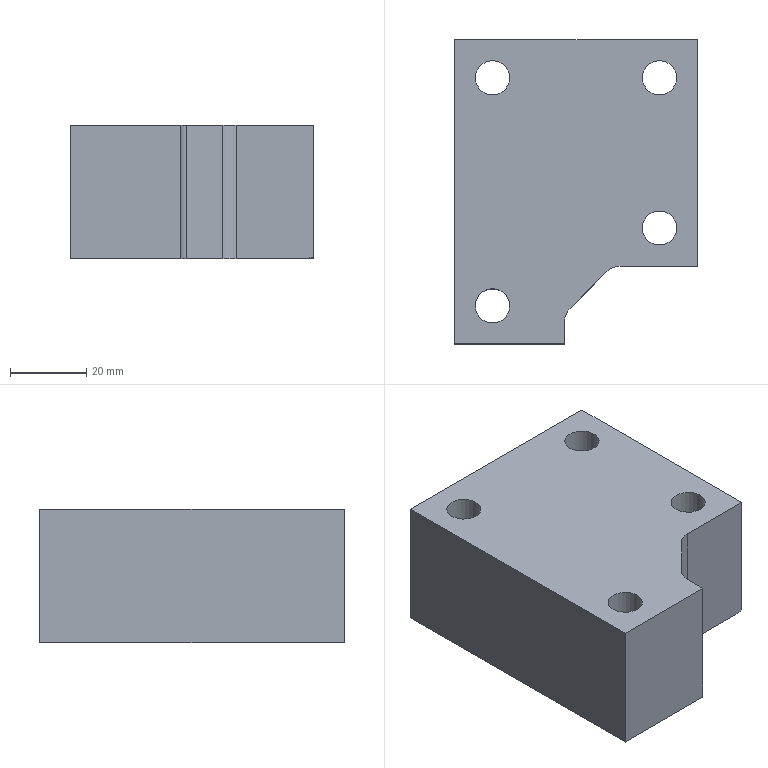Part | STEP file | PN_0033_id754_x_t | 1 solid | 56 faces | box 63.914 x 80 x 35 mm | volume 137778 mm3 | spline 30 | plane 14 | cylinder 10 | torus 1 | sphere 1 | commonest cylinder face diameters 9 x4 14 x4 10 x2